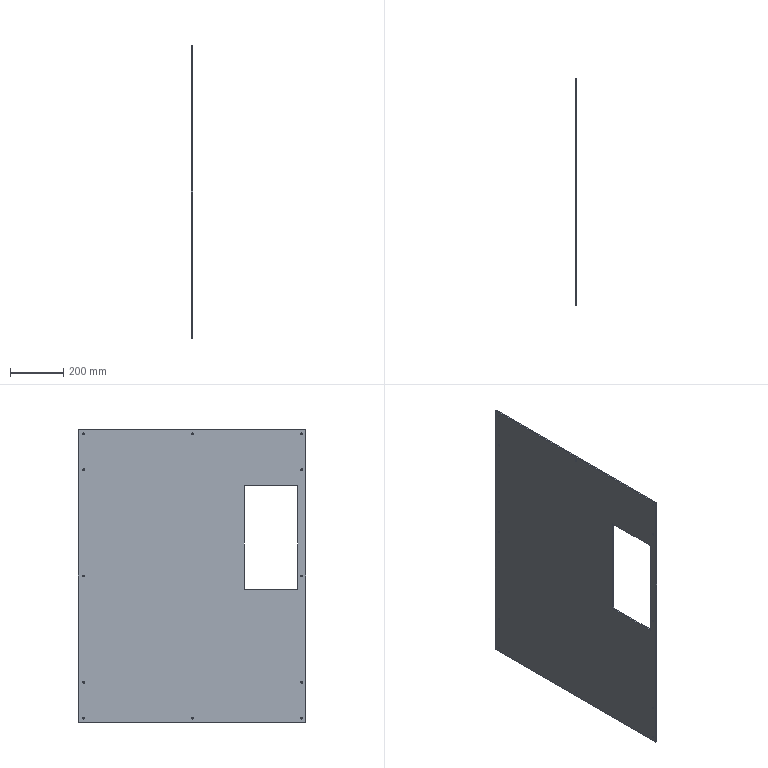Part | STEP file | 08-08 Seal plate | 1 solid | 34 faces | box 5 x 855 x 1100 mm | volume 4310509 mm3 | cylinder 24 | plane 10 | commonest cylinder face diameters 6.5 x24